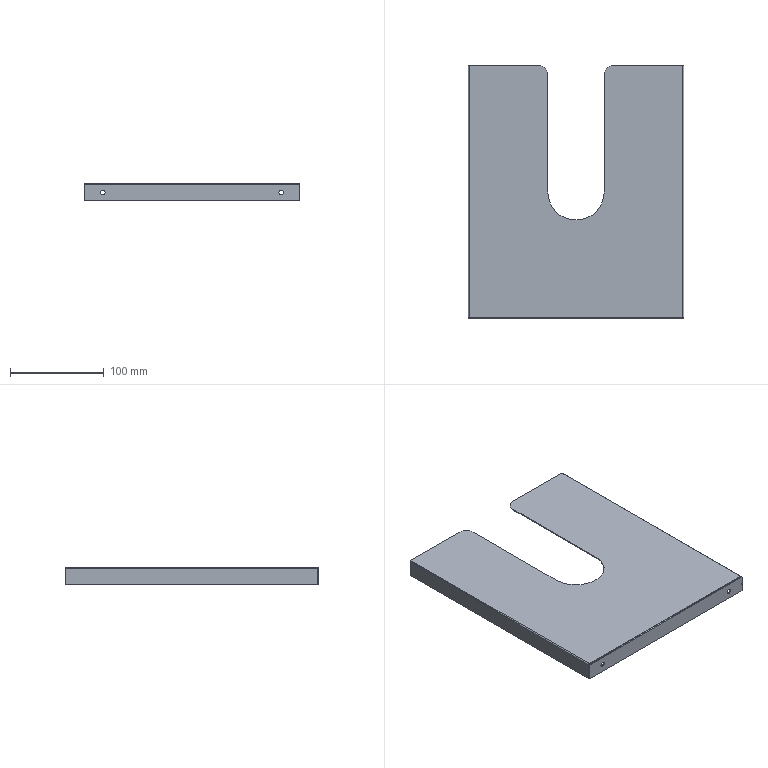Part | STEP file | 1 solid | 40 faces | box 230 x 270 x 19 mm | volume 66126 mm3 | plane 25 | cylinder 13 | spline 2 | commonest cylinder face diameters 5 x4 0.2 x3 2.2 x3 20 x2 60 x1